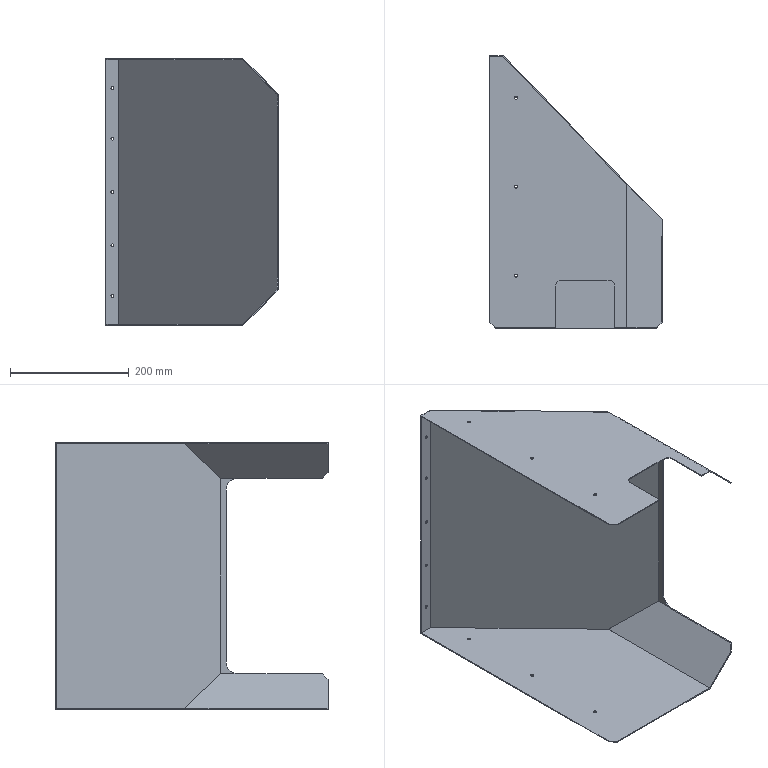Part | SolidWorks | features ICE 3, Chamfer 2, Fillet 2, HoleWzd 2, Cut 1, Extrusion 1, Shell 1 | 1 solid | 54 faces | box 291.379 x 459 x 450 mm | volume 562912 mm3 | plane 28 | cylinder 26 | commonest cylinder face diameters 5 x22 20 x2 40 x2